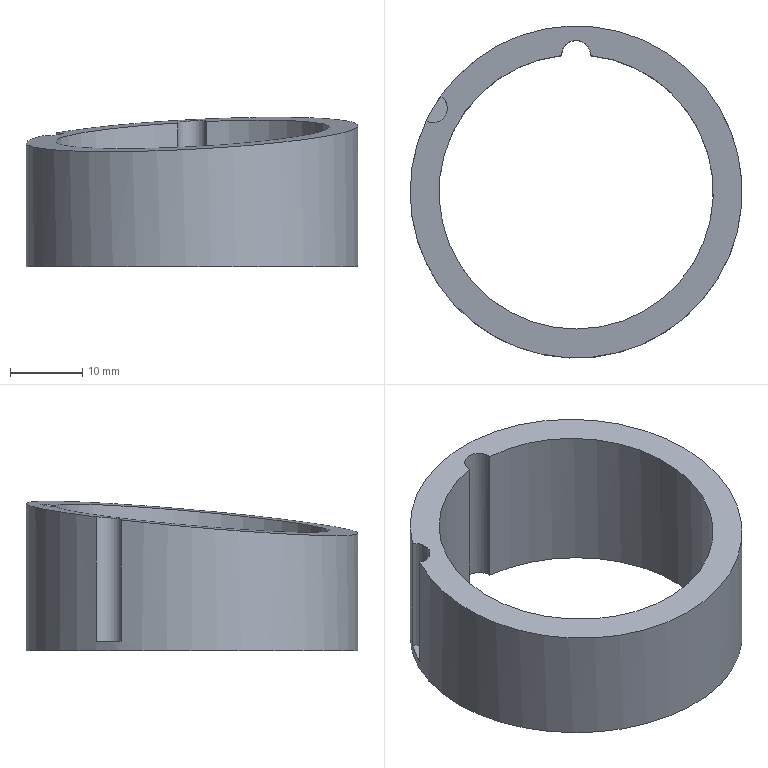Part | NX | features solid 2 | 1 solid | 7 faces | box 46 x 46 x 20.725 mm | volume 9446 mm3 | cylinder 4 | plane 3 | commonest cylinder face diameters 4 x2 38 x1 46 x1
STEP:
#1=CARTESIAN_POINT('',(-192.893,7.418,-4.073));
#2=VERTEX_POINT('',#1);
#3=CARTESIAN_POINT('',(-188.899,7.418,-3.864));
#4=VERTEX_POINT('',#3);
#5=CARTESIAN_POINT('',(-190.896,-11.477,-5.66));
#6=DIRECTION('',(0.05204,0.08903,-0.9947));
#7=DIRECTION('',(-0.502,-0.8587,-0.1031));
#8=AXIS2_PLACEMENT_3D('',#5,#6,#7);
#9=ELLIPSE('',#8,19.102,19.);
#10=EDGE_CURVE('',#2,#4,#9,.F.);
#11=ORIENTED_EDGE('',*,*,#10,.T.);
#12=CARTESIAN_POINT('',(-188.899,7.418,-24.));
#13=VERTEX_POINT('',#12);
#14=CARTESIAN_POINT('',(-188.899,7.418,-13.815));
#15=DIRECTION('',(0.,0.,-1.));
#16=VECTOR('',#15,1000.);
#17=LINE('',#14,#16);
#18=EDGE_CURVE('',#4,#13,#17,.T.);
#19=ORIENTED_EDGE('',*,*,#18,.T.);
#20=CARTESIAN_POINT('',(-192.893,7.418,-24.));
#21=VERTEX_POINT('',#20);
#22=CARTESIAN_POINT('',(-190.896,-11.477,-24.));
#23=DIRECTION('',(0.,0.,-1.));
#24=DIRECTION('',(-1.,0.,0.));
#25=AXIS2_PLACEMENT_3D('',#22,#23,#24);
#26=CIRCLE('',#25,19.);
#27=EDGE_CURVE('',#21,#13,#26,.F.);
#28=ORIENTED_EDGE('',*,*,#27,.F.);
#29=CARTESIAN_POINT('',(-192.893,7.418,-13.815));
#30=DIRECTION('',(0.,0.,-1.));
#31=VECTOR('',#30,1000.);
#32=LINE('',#29,#31);
#33=EDGE_CURVE('',#21,#2,#32,.F.);
#34=ORIENTED_EDGE('',*,*,#33,.T.);
#35=EDGE_LOOP('',(#11,#19,#28,#34));
#36=FACE_BOUND('',#35,.T.);
#37=CARTESIAN_POINT('',(-190.896,-11.477,-3.5));
#38=DIRECTION('',(0.,0.,-1.));
#39=DIRECTION('',(-1.,0.,0.));
#40=AXIS2_PLACEMENT_3D('',#37,#38,#39);
#41=CYLINDRICAL_SURFACE('',#40,19.);
#42=ADVANCED_FACE('',(#36),#41,.F.);
#43=CARTESIAN_POINT('',(-190.896,7.523,-24.));
#44=DIRECTION('',(0.,0.,-1.));
#45=DIRECTION('',(-1.,0.,0.));
#46=AXIS2_PLACEMENT_3D('',#43,#44,#45);
#47=CIRCLE('',#46,2.);
#48=EDGE_CURVE('',#13,#21,#47,.F.);
#49=ORIENTED_EDGE('',*,*,#48,.T.);
#50=ORIENTED_EDGE('',*,*,#27,.T.);
#51=EDGE_LOOP('',(#49,#50));
#52=FACE_BOUND('',#51,.T.);
#53=CARTESIAN_POINT('',(-213.896,-11.477,-24.));
#54=VERTEX_POINT('',#53);
#55=CARTESIAN_POINT('',(-190.896,-11.477,-24.));
#56=DIRECTION('',(0.,0.,-1.));
#57=DIRECTION('',(-1.,0.,0.));
#58=AXIS2_PLACEMENT_3D('',#55,#56,#57);
#59=CIRCLE('',#58,23.);
#60=EDGE_CURVE('',#54,#54,#59,.F.);
#61=ORIENTED_EDGE('',*,*,#60,.F.);
#62=EDGE_LOOP('',(#61));
#63=FACE_BOUND('',#62,.T.);
#64=CARTESIAN_POINT('',(-190.896,-11.477,-24.));
#65=DIRECTION('',(0.,0.,-1.));
#66=DIRECTION('',(-1.,0.,0.));
#67=AXIS2_PLACEMENT_3D('',#64,#65,#66);
#68=PLANE('',#67);
#69=ADVANCED_FACE('',(#52,#63),#68,.T.);
#70=CARTESIAN_POINT('',(-190.896,7.523,-3.959));
#71=DIRECTION('',(0.05204,0.08903,-0.9947));
#72=DIRECTION('',(-0.502,-0.8587,-0.1031));
#73=AXIS2_PLACEMENT_3D('',#70,#71,#72);
#74=ELLIPSE('',#73,2.011,2.);
#75=EDGE_CURVE('',#2,#4,#74,.T.);
#76=ORIENTED_EDGE('',*,*,#75,.T.);
#77=ORIENTED_EDGE('',*,*,#10,.F.);
#78=EDGE_LOOP('',(#76,#77));
#79=FACE_BOUND('',#78,.T.);
#80=CARTESIAN_POINT('',(-209.669,1.811,-5.452));
#81=VERTEX_POINT('',#80);
#82=CARTESIAN_POINT('',(-211.686,-1.639,-5.867));
#83=VERTEX_POINT('',#82);
#84=CARTESIAN_POINT('',(-210.753,0.1299,-5.66));
#85=DIRECTION('',(0.05204,0.08903,-0.9947));
#86=DIRECTION('',(-0.502,-0.8587,-0.1031));
#87=AXIS2_PLACEMENT_3D('',#84,#85,#86);
#88=ELLIPSE('',#87,2.011,2.);
#89=EDGE_CURVE('',#81,#83,#88,.T.);
#90=ORIENTED_EDGE('',*,*,#89,.T.);
#91=CARTESIAN_POINT('',(-190.896,-11.477,-5.66));
#92=DIRECTION('',(0.05204,0.08903,-0.9947));
#93=DIRECTION('',(-0.502,-0.8587,-0.1031));
#94=AXIS2_PLACEMENT_3D('',#91,#92,#93);
#95=ELLIPSE('',#94,23.123,23.);
#96=EDGE_CURVE('',#83,#81,#95,.F.);
#97=ORIENTED_EDGE('',*,*,#96,.T.);
#98=EDGE_LOOP('',(#90,#97));
#99=FACE_BOUND('',#98,.T.);
#100=CARTESIAN_POINT('',(-99.272,-11.445,-0.8629));
#101=DIRECTION('',(0.05204,0.08903,-0.9947));
#102=DIRECTION('',(0.005002,-0.996,-0.08889));
#103=AXIS2_PLACEMENT_3D('',#100,#101,#102);
#104=PLANE('',#103);
#105=ADVANCED_FACE('',(#79,#99),#104,.F.);
#106=CARTESIAN_POINT('',(-211.686,-1.639,-22.666));
#107=VERTEX_POINT('',#106);
#108=CARTESIAN_POINT('',(-209.669,1.811,-22.666));
#109=VERTEX_POINT('',#108);
#110=CARTESIAN_POINT('',(-190.896,-11.477,-22.666));
#111=DIRECTION('',(0.,0.,-1.));
#112=DIRECTION('',(-1.,0.,0.));
#113=AXIS2_PLACEMENT_3D('',#110,#111,#112);
#114=CIRCLE('',#113,23.);
#115=EDGE_CURVE('',#107,#109,#114,.T.);
#116=ORIENTED_EDGE('',*,*,#115,.T.);
#117=CARTESIAN_POINT('',(-209.669,1.811,-14.008));
#118=DIRECTION('',(0.,0.,-1.));
#119=VECTOR('',#118,1000.);
#120=LINE('',#117,#119);
#121=EDGE_CURVE('',#109,#81,#120,.F.);
#122=ORIENTED_EDGE('',*,*,#121,.T.);
#123=ORIENTED_EDGE('',*,*,#96,.F.);
#124=CARTESIAN_POINT('',(-211.686,-1.639,-14.008));
#125=DIRECTION('',(0.,0.,-1.));
#126=VECTOR('',#125,1000.);
#127=LINE('',#124,#126);
#128=EDGE_CURVE('',#83,#107,#127,.T.);
#129=ORIENTED_EDGE('',*,*,#128,.T.);
#130=EDGE_LOOP('',(#116,#122,#123,#129));
#131=FACE_BOUND('',#130,.T.);
#132=ORIENTED_EDGE('',*,*,#60,.T.);
#133=EDGE_LOOP('',(#132));
#134=FACE_BOUND('',#133,.T.);
#135=CARTESIAN_POINT('',(-190.896,-11.477,-3.5));
#136=DIRECTION('',(0.,0.,-1.));
#137=DIRECTION('',(-1.,0.,0.));
#138=AXIS2_PLACEMENT_3D('',#135,#136,#137);
#139=CYLINDRICAL_SURFACE('',#138,23.);
#140=ADVANCED_FACE('',(#131,#134),#139,.T.);
#141=CARTESIAN_POINT('',(-210.753,0.1299,-22.666));
#142=DIRECTION('',(0.,0.,1.));
#143=DIRECTION('',(1.,0.,0.));
#144=AXIS2_PLACEMENT_3D('',#141,#142,#143);
#145=CIRCLE('',#144,2.);
#146=EDGE_CURVE('',#107,#109,#145,.T.);
#147=ORIENTED_EDGE('',*,*,#146,.T.);
#148=ORIENTED_EDGE('',*,*,#115,.F.);
#149=EDGE_LOOP('',(#147,#148));
#150=FACE_BOUND('',#149,.T.);
#151=CARTESIAN_POINT('',(-210.753,0.1299,-22.666));
#152=DIRECTION('',(0.,0.,-1.));
#153=DIRECTION('',(-1.,0.,0.));
#154=AXIS2_PLACEMENT_3D('',#151,#152,#153);
#155=PLANE('',#154);
#156=ADVANCED_FACE('',(#150),#155,.F.);
#157=ORIENTED_EDGE('',*,*,#146,.F.);
#158=ORIENTED_EDGE('',*,*,#128,.F.);
#159=ORIENTED_EDGE('',*,*,#89,.F.);
#160=ORIENTED_EDGE('',*,*,#121,.F.);
#161=EDGE_LOOP('',(#157,#158,#159,#160));
#162=FACE_BOUND('',#161,.T.);
#163=CARTESIAN_POINT('',(-210.753,0.1299,-2.666));
#164=DIRECTION('',(0.,0.,-1.));
#165=DIRECTION('',(-1.,0.,0.));
#166=AXIS2_PLACEMENT_3D('',#163,#164,#165);
#167=CYLINDRICAL_SURFACE('',#166,2.);
#168=ADVANCED_FACE('',(#162),#167,.F.);
#169=ORIENTED_EDGE('',*,*,#75,.F.);
#170=ORIENTED_EDGE('',*,*,#33,.F.);
#171=ORIENTED_EDGE('',*,*,#48,.F.);
#172=ORIENTED_EDGE('',*,*,#18,.F.);
#173=EDGE_LOOP('',(#169,#170,#171,#172));
#174=FACE_BOUND('',#173,.T.);
#175=CARTESIAN_POINT('',(-190.896,7.523,-3.5));
#176=DIRECTION('',(0.,0.,-1.));
#177=DIRECTION('',(-1.,0.,0.));
#178=AXIS2_PLACEMENT_3D('',#175,#176,#177);
#179=CYLINDRICAL_SURFACE('',#178,2.);
#180=ADVANCED_FACE('',(#174),#179,.F.);
#181=CLOSED_SHELL('',(#42,#69,#105,#140,#156,#168,#180));
#182=MANIFOLD_SOLID_BREP('',#181);
#183=(LENGTH_UNIT()NAMED_UNIT(*)SI_UNIT(.MILLI.,.METRE.));
#184=UNCERTAINTY_MEASURE_WITH_UNIT(LENGTH_MEASURE(0.00001),#183,'','');
#185=(NAMED_UNIT(*)PLANE_ANGLE_UNIT()SI_UNIT($,.RADIAN.));
#186=(NAMED_UNIT(*)SI_UNIT($,.STERADIAN.)SOLID_ANGLE_UNIT());
#187=(GEOMETRIC_REPRESENTATION_CONTEXT(3)GLOBAL_UNCERTAINTY_ASSIGNED_CONTEXT((#184))GLOBAL_UNIT_ASSIGNED_CONTEXT((#183,#185,#186))REPRESENTATION_CONTEXT('',''));
#188=ADVANCED_BREP_SHAPE_REPRESENTATION('',(#182),#187);